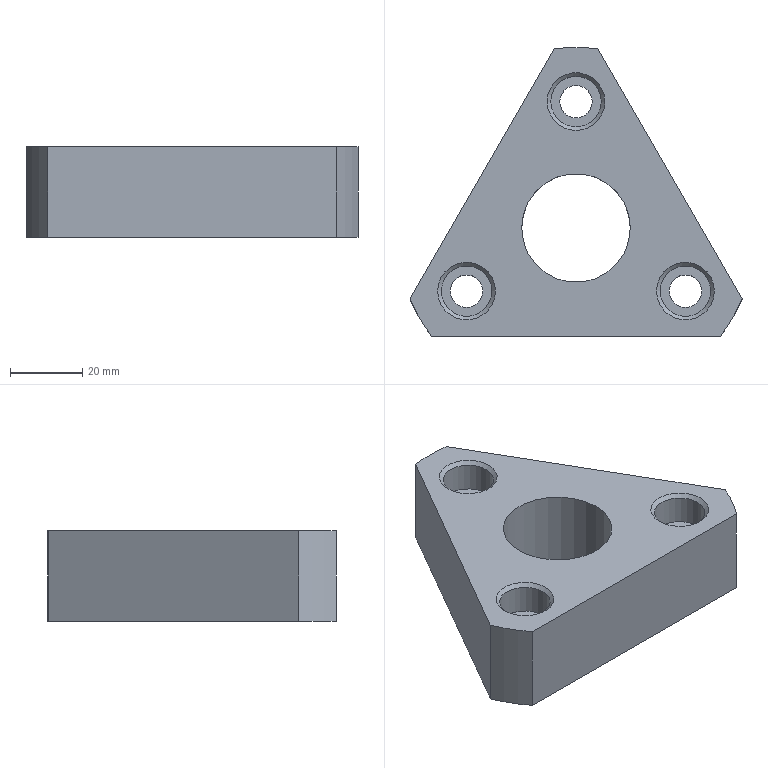NC program | NX | posted with a generic post | part box 91.962 x 80 x 25 mm
Lines 829 to 1659 of 11626:
(ZLEVEL_PROFILE_COPY , TOOL : D25R0.8)
N1632 T01 M6
N1634 G54
N1636 G17 G0 G90 X-0.726 Y-12.359 S1600 M3
N1638 G43 Z30. H1
N1640 Z1.
N1642 G94 G1 X-0.554 Y-12.412 Z0.991 F1000.
N1644 X-0.176 Y-12.436 Z0.971
N1646 X-0.153 Y-12.445 Z0.969
N1648 X-0.141 Y-12.441
N1650 X0.128 Z0.955
N1652 X0.136 Y-12.446 Z0.954
N1654 X0.157 Y-12.436 Z0.953
N1656 X0.354 Y-12.417 Z0.943
N1658 X1.218 Y-12.12 Z0.895
N1660 X2.118 Y-11.218 Z0.828
N1662 X2.308 Y-10.893 Z0.808
N1664 X2.414 Y-10.542 Z0.789
N1666 X2.436 Y-10.166 Z0.769
N1668 X2.446 Y-10.141 Z0.768
N1670 Y-9.859 Z0.753
N1672 X2.436 Y-9.839 Z0.752
N1674 X2.417 Y-9.644 Z0.742
N1676 X2.118 Y-8.782 Z0.694
N1678 X1.218 Y-7.88 Z0.627
N1680 X0.89 Y-7.69 Z0.607
N1682 X0.515 Y-7.581 Z0.587
N1684 X0.136 Y-7.563 Z0.567
N1686 Y-7.554 Z0.566
N1688 X0.128 Y-7.559
N1690 X-0.153 Y-7.555 Z0.551
N1692 X-0.171 Y-7.564 Z0.55
N1694 X-0.548 Y-7.587 Z0.53
N1696 X-0.892 Y-7.692 Z0.511
N1698 X-1.218 Y-7.882 Z0.492
N1700 X-2.118 Y-8.782 Z0.425
N1702 X-2.308 Y-9.105 Z0.405
N1704 X-2.419 Y-9.478 Z0.385
N1706 X-2.437 Y-9.852 Z0.365
N1708 X-2.446
N1710 Y-10.148 Z0.349
N1712 X-2.436 Y-10.167 Z0.348
N1714 X-2.414 Y-10.543 Z0.328
N1716 X-2.308 Y-10.893 Z0.309
N1718 X-2.118 Y-11.218 Z0.289
N1720 X-1.218 Y-12.118 Z0.223
N1722 X-0.892 Y-12.309 Z0.203
N1724 X-0.554 Y-12.412 Z0.184
N1726 X-0.176 Y-12.436 Z0.165
N1728 X-0.153 Y-12.445 Z0.163
N1730 X-0.141 Y-12.441
N1732 X0.128 Z0.149
N1734 X0.136 Y-12.446 Z0.148
N1736 X0.157 Y-12.436 Z0.147
N1738 X0.354 Y-12.417 Z0.137
N1740 X1.218 Y-12.12 Z0.089
N1742 X2.118 Y-11.218 Z0.022
N1744 X2.308 Y-10.893 Z0.002
N1746 X2.414 Y-10.542 Z-0.017
N1748 X2.436 Y-10.166 Z-0.037
N1750 X2.446 Y-10.141 Z-0.038
N1752 Y-9.859 Z-0.053
N1754 X2.436 Y-9.839 Z-0.054
N1756 X2.417 Y-9.644 Z-0.064
N1758 X2.118 Y-8.782 Z-0.112
N1760 X1.218 Y-7.88 Z-0.179
N1762 X0.89 Y-7.69 Z-0.199
N1764 X0.515 Y-7.581 Z-0.219
N1766 X0.136 Y-7.563 Z-0.239
N1768 Y-7.554 Z-0.24
N1770 X0.128 Y-7.559
N1772 X-0.153 Y-7.555 Z-0.255
N1774 X-0.171 Y-7.564 Z-0.256
N1776 X-0.548 Y-7.587 Z-0.276
N1778 X-0.892 Y-7.692 Z-0.295
N1780 X-1.218 Y-7.882 Z-0.314
N1782 X-1.668 Y-8.332 Z-0.348
N1784 X-2.118 Y-8.782 F1800.
N1786 G3 X-2.437 Y-9.852 R2.327
N1788 G1 X-2.446
N1790 Y-10.148
N1792 X-2.436 Y-10.167
N1794 G3 X-2.118 Y-11.218 R2.352
N1796 G1 X-1.218 Y-12.118
N1798 G3 X-0.176 Y-12.436 R2.371
N1800 G1 X-0.153 Y-12.445
N1802 X-0.141 Y-12.441
N1804 X0.128
N1806 X0.136 Y-12.446
N1808 X0.157 Y-12.436
N1810 X0.354 Y-12.417
N1812 X1.218 Y-12.12
N1814 X2.118 Y-11.218
N1816 G3 X2.436 Y-10.166 R2.356
N1818 G1 X2.446 Y-10.141
N1820 Y-9.859
N1822 X2.436 Y-9.839
N1824 X2.417 Y-9.644
N1826 X2.118 Y-8.782
N1828 X1.218 Y-7.88
N1830 G3 X0.136 Y-7.563 R2.383
N1832 G1 Y-7.554
N1834 X0.128 Y-7.559
N1836 X-0.153 Y-7.555
N1838 X-0.171 Y-7.564
N1840 G3 X-1.218 Y-7.882 R2.363
N1842 G1 X-1.668 Y-8.332
N1844 X-2.101 Y-8.765 Z-0.362
N1846 X-2.349 Y-9.322 Z-0.376
N1848 X-2.446 Y-9.917 Z-0.39
N1850 X-2.388 Y-10.524 Z-0.403
N1852 X-2.183 Y-11.1 Z-0.417
N1854 X-1.78 Y-11.556 Z-0.431
N1856 X-1.347 Y-11.989 Z-0.445
N1858 X-0.829 Y-12.3 Z-0.459
N1860 X-0.232 Y-12.432 Z-0.473
N1862 X0.373 Y-12.411 Z-0.487
N1864 X0.952 Y-12.212 Z-0.501
N1866 X1.452 Y-11.886 Z-0.515
N1868 X1.885 Y-11.452 Z-0.529
N1870 X2.246 Y-10.966 Z-0.543
N1872 X2.414 Y-10.379 Z-0.557
N1874 X2.43 Y-9.772 Z-0.57
N1876 X2.259 Y-9.187 Z-0.584
N1878 X1.988 Y-8.652 Z-0.598
N1880 X1.555 Y-8.218 Z-0.612
N1882 X1.099 Y-7.815 Z-0.626
N1884 X0.523 Y-7.613 Z-0.64
N1886 X-0.076 Y-7.556 Z-0.654
N1888 X-0.678 Y-7.651 Z-0.668
N1890 X-1.235 Y-7.899 Z-0.682
N1892 X-1.668 Y-8.332 Z-0.696
N1894 X-2.118 Y-8.782
N1896 G3 X-2.437 Y-9.852 R2.327
N1898 G1 X-2.446
N1900 Y-10.148
N1902 X-2.436 Y-10.167
N1904 G3 X-2.118 Y-11.218 R2.352
N1906 G1 X-1.218 Y-12.118
N1908 G3 X-0.176 Y-12.436 R2.371
N1910 G1 X-0.153 Y-12.445
N1912 X-0.141 Y-12.441
N1914 X0.128
N1916 X0.136 Y-12.446
N1918 X0.157 Y-12.436
N1920 X0.354 Y-12.417
N1922 X1.218 Y-12.12
N1924 X2.118 Y-11.218
N1926 G3 X2.436 Y-10.166 R2.356
N1928 G1 X2.446 Y-10.141
N1930 Y-9.859
N1932 X2.436 Y-9.839
N1934 X2.417 Y-9.644
N1936 X2.118 Y-8.782
N1938 X1.218 Y-7.88
N1940 G3 X0.136 Y-7.563 R2.383
N1942 G1 Y-7.554
N1944 X0.128 Y-7.559
N1946 X-0.153 Y-7.555
N1948 X-0.171 Y-7.564
N1950 G3 X-1.218 Y-7.882 R2.363
N1952 G1 X-1.668 Y-8.332
N1954 Z0.304
N1956 G0 X-0.553 Y-12.416
N1958 G1 X-0.153 Y-12.445 Z0.283 F1000.
N1960 X0.231 Y-12.469 Z0.263
N1962 X1.213 Y-12.163 Z0.209
N1964 X1.987 Y-11.484 Z0.155
N1966 X2.418 Y-10.55 Z0.101
N1968 X2.446 Y-10.141 Z0.08
N1970 X2.454 Y-10. Z0.073
N1972 X2.445 Y-9.838 Z0.064
N1974 X2.419 Y-9.455 Z0.044
N1976 X2.046 Y-8.598 Z-0.005
N1978 X1.381 Y-7.94 Z-0.054
N1980 X0.521 Y-7.575 Z-0.103
N1982 X0.136 Y-7.554 Z-0.123
N1984 X-0.008 Y-7.546 Z-0.131
N1986 X-0.172 Y-7.556 Z-0.139
N1988 X-0.555 Y-7.583 Z-0.16
N1990 X-1.46 Y-7.996 Z-0.212
N1992 X-2.004 Y-8.54 Z-0.252
N1994 X-2.422 Y-9.468 Z-0.305
N1996 X-2.446 Y-9.852 Z-0.326
N1998 X-2.454 Y-10. Z-0.333
N2000 X-2.444 Y-10.168 Z-0.342
N2002 X-2.418 Y-10.551 Z-0.362
N2004 X-2.051 Y-11.394 Z-0.41
N2006 X-1.402 Y-12.046 Z-0.459
N2008 X-0.56 Y-12.416 Z-0.507
N2010 X-0.153 Y-12.445 Z-0.528
N2012 X0.231 Y-12.469 Z-0.548
N2014 X1.213 Y-12.163 Z-0.602
N2016 X1.987 Y-11.484 Z-0.656
N2018 X2.418 Y-10.55 Z-0.71
N2020 X2.446 Y-10.141 Z-0.732
N2022 X2.454 Y-10. Z-0.739
N2024 X2.445 Y-9.838 Z-0.748
N2026 X2.419 Y-9.455 Z-0.768
N2028 X2.046 Y-8.598 Z-0.817
N2030 X1.381 Y-7.94 Z-0.866
N2032 X0.521 Y-7.575 Z-0.915
N2034 X0.136 Y-7.554 Z-0.935
N2036 X-0.008 Y-7.546 Z-0.942
N2038 X-0.172 Y-7.556 Z-0.951
N2040 X-0.555 Y-7.583 Z-0.971
N2042 X-1.46 Y-7.996 Z-1.023
N2044 X-1.732 Y-8.268 Z-1.043
N2046 G3 X-1.732 Y-11.732 R2.45 F1800.
N2048 X-1.732 Y-8.268 R-2.45
N2050 G1 X-1.963 Y-8.549 Z-1.052
N2052 X-2.088 Y-8.737 Z-1.057
N2054 X-2.25 Y-9.055 Z-1.065
N2056 X-2.332 Y-9.273 Z-1.07
N2058 X-2.402 Y-9.567 Z-1.077
N2060 X-2.438 Y-9.852 Z-1.084
N2062 X-2.442 Y-10.045 Z-1.088
N2064 X-2.437 Y-10.164 Z-1.091
N2066 X-2.368 Y-10.598 Z-1.101
N2068 X-2.291 Y-10.848 Z-1.107
N2070 X-2.115 Y-11.221 Z-1.116
N2072 X-1.958 Y-11.46 Z-1.122
N2074 X-1.688 Y-11.764 Z-1.132
N2076 X-1.467 Y-11.953 Z-1.138
N2078 X-1.121 Y-12.169 Z-1.148
N2080 X-0.856 Y-12.288 Z-1.154
N2082 X-0.445 Y-12.402 Z-1.164
N2084 X-0.152 Y-12.438 Z-1.17
N2086 X0.15 Z-1.177
N2088 X0.3 Y-12.423 Z-1.181
N2090 X0.402 Y-12.409 Z-1.183
N2092 X0.606 Y-12.366 Z-1.188
N2094 X0.897 Y-12.273 Z-1.195
N2096 X1.036 Y-12.212 Z-1.198
N2098 X1.127 Y-12.165 Z-1.2
N2100 X1.304 Y-12.063 Z-1.205
N2102 X1.559 Y-11.877 Z-1.212
N2104 X1.678 Y-11.774 Z-1.216
N2106 X1.747 Y-11.707 Z-1.218
N2108 X1.878 Y-11.562 Z-1.222
N2110 X2.14 Y-11.172 Z-1.233
N2112 X2.267 Y-10.908 Z-1.24
N2114 X2.348 Y-10.665 Z-1.246
N2116 X2.381 Y-10.54 Z-1.248
N2118 X2.407 Y-10.409 Z-1.252
N2120 X2.439 Y-10.141 Z-1.258
N2122 X2.446 Y-9.96 Z-1.262
N2124 X2.439 Y-9.859 Z-1.264
N2126 X2.362 Y-9.376 Z-1.275
N2128 X2.287 Y-9.15 Z-1.281
N2130 X2.103 Y-8.759 Z-1.29
N2132 X1.949 Y-8.532 Z-1.297
N2134 X1.669 Y-8.218 Z-1.306
N2136 X1.448 Y-8.036 Z-1.313
N2138 X1.092 Y-7.817 Z-1.322
N2140 X0.827 Y-7.704 Z-1.329
N2142 X0.619 Y-7.629 Z-1.334
N2144 X0.512 Y-7.604 Z-1.336
N2146 X0.387 Y-7.589 Z-1.339
N2148 X0.136 Y-7.564 Z-1.345
N2150 X-0.016 Y-7.56 Z-1.348
N2152 X-0.169 Y-7.556 Z-1.352
N2154 X-0.449 Y-7.6 Z-1.358
N2156 X-0.741 Y-7.675 Z-1.365
N2158 X-1.05 Y-7.797 Z-1.372
N2160 X-1.27 Y-7.914 Z-1.378
N2162 X-1.509 Y-8.082 Z-1.385
N2164 X-1.732 Y-8.268 Z-1.391
N2166 X-1.963 Y-8.549 Z-1.4
N2168 X-2.088 Y-8.737 Z-1.405
N2170 X-2.25 Y-9.055 Z-1.413
N2172 X-2.332 Y-9.273 Z-1.418
N2174 X-2.402 Y-9.567 Z-1.425
N2176 X-2.438 Y-9.852 Z-1.431
N2178 X-2.442 Y-10.045 Z-1.436
N2180 X-2.437 Y-10.164 Z-1.439
N2182 X-2.368 Y-10.598 Z-1.449
N2184 X-2.291 Y-10.848 Z-1.454
N2186 X-2.115 Y-11.221 Z-1.464
N2188 X-1.958 Y-11.46 Z-1.47
N2190 X-1.688 Y-11.764 Z-1.479
N2192 X-1.467 Y-11.953 Z-1.486
N2194 X-1.121 Y-12.169 Z-1.495
N2196 X-0.856 Y-12.288 Z-1.502
N2198 X-0.445 Y-12.402 Z-1.512
N2200 X-0.152 Y-12.438 Z-1.518
N2202 X0.15 Z-1.525
N2204 X0.3 Y-12.423 Z-1.529
N2206 X0.402 Y-12.409 Z-1.531
N2208 X0.606 Y-12.366 Z-1.536
N2210 X0.897 Y-12.273 Z-1.543
N2212 X1.036 Y-12.212 Z-1.546
N2214 X1.127 Y-12.165 Z-1.548
N2216 X1.304 Y-12.063 Z-1.553
N2218 X1.559 Y-11.877 Z-1.56
N2220 X1.678 Y-11.774 Z-1.564
N2222 X1.747 Y-11.707 Z-1.566
N2224 X1.878 Y-11.562 Z-1.57
N2226 X2.14 Y-11.172 Z-1.581
N2228 X2.267 Y-10.908 Z-1.588
N2230 X2.348 Y-10.665 Z-1.593
N2232 X2.381 Y-10.54 Z-1.596
N2234 X2.407 Y-10.409 Z-1.599
N2236 X2.439 Y-10.141 Z-1.605
N2238 X2.446 Y-9.96 Z-1.61
N2240 X2.439 Y-9.859 Z-1.612
N2242 X2.362 Y-9.376 Z-1.623
N2244 X2.287 Y-9.15 Z-1.628
N2246 X2.103 Y-8.759 Z-1.638
N2248 X1.949 Y-8.532 Z-1.644
N2250 X1.669 Y-8.218 Z-1.654
N2252 X1.448 Y-8.036 Z-1.66
N2254 X1.092 Y-7.817 Z-1.67
N2256 X0.827 Y-7.704 Z-1.676
N2258 X0.619 Y-7.629 Z-1.681
N2260 X0.512 Y-7.604 Z-1.684
N2262 X0.387 Y-7.589 Z-1.687
N2264 X0.136 Y-7.564 Z-1.693
N2266 X-0.016 Y-7.56 Z-1.696
N2268 X-0.169 Y-7.556 Z-1.699
N2270 X-0.449 Y-7.6 Z-1.706
N2272 X-0.741 Y-7.675 Z-1.713
N2274 X-1.05 Y-7.797 Z-1.72
N2276 X-1.27 Y-7.914 Z-1.726
N2278 X-1.509 Y-8.082 Z-1.733
N2280 X-1.732 Y-8.268 Z-1.739
N2282 X-1.963 Y-8.549 Z-1.747
N2284 X-2.088 Y-8.737 Z-1.753
N2286 X-2.25 Y-9.055 Z-1.761
N2288 X-2.332 Y-9.273 Z-1.766
N2290 X-2.402 Y-9.567 Z-1.773
N2292 X-2.438 Y-9.852 Z-1.779
N2294 X-2.442 Y-10.045 Z-1.784
N2296 X-2.437 Y-10.164 Z-1.786
N2298 X-2.368 Y-10.598 Z-1.796
N2300 X-2.291 Y-10.848 Z-1.802
N2302 X-2.115 Y-11.221 Z-1.812
N2304 X-1.958 Y-11.46 Z-1.818
N2306 X-1.688 Y-11.764 Z-1.827
N2308 X-1.467 Y-11.953 Z-1.834
N2310 X-1.121 Y-12.169 Z-1.843
N2312 X-0.856 Y-12.288 Z-1.85
N2314 X-0.445 Y-12.402 Z-1.859
N2316 X-0.152 Y-12.438 Z-1.866
N2318 X0.15 Z-1.873
N2320 X0.3 Y-12.423 Z-1.876
N2322 X0.402 Y-12.409 Z-1.879
N2324 X0.606 Y-12.366 Z-1.883
N2326 X0.897 Y-12.273 Z-1.89
N2328 X1.036 Y-12.212 Z-1.894
N2330 X1.127 Y-12.165 Z-1.896
N2332 X1.304 Y-12.063 Z-1.901
N2334 X1.559 Y-11.877 Z-1.908
N2336 X1.678 Y-11.774 Z-1.911
N2338 X1.747 Y-11.707 Z-1.914
N2340 X1.878 Y-11.562 Z-1.918
N2342 X2.14 Y-11.172 Z-1.929
N2344 X2.267 Y-10.908 Z-1.935
N2346 X2.348 Y-10.665 Z-1.941
N2348 X2.381 Y-10.54 Z-1.944
N2350 X2.407 Y-10.409 Z-1.947
N2352 X2.439 Y-10.141 Z-1.953
N2354 X2.445 Y-9.96 Z-1.957
N2356 X2.439 Y-9.859 Z-1.96
N2358 X2.362 Y-9.376 Z-1.971
N2360 X2.287 Y-9.15 Z-1.976
N2362 X2.103 Y-8.759 Z-1.986
N2364 X1.949 Y-8.532 Z-1.992
N2366 X1.669 Y-8.218 Z-2.002
N2368 X1.448 Y-8.036 Z-2.008
N2370 X1.092 Y-7.817 Z-2.018
N2372 X0.827 Y-7.704 Z-2.024
N2374 X0.619 Y-7.629 Z-2.029
N2376 X0.389 Y-7.581 Z-2.035
N2378 X0.136 Y-7.564 Z-2.04
N2380 X-0.017 Y-7.55 Z-2.044
N2382 X-0.169 Y-7.556 Z-2.047
N2384 X-0.497 Y-7.601 Z-2.055
N2386 X-0.741 Y-7.675 Z-2.061
N2388 X-1.087 Y-7.813 Z-2.069
N2390 X-1.27 Y-7.914 Z-2.074
N2392 X-1.509 Y-8.082 Z-2.08
N2394 X-1.732 Y-8.268 Z-2.087
N2396 X-1.963 Y-8.549 Z-2.095
N2398 X-2.088 Y-8.737 Z-2.1
N2400 X-2.25 Y-9.055 Z-2.108
N2402 X-2.332 Y-9.273 Z-2.114
N2404 X-2.402 Y-9.567 Z-2.121
N2406 X-2.438 Y-9.852 Z-2.127
N2408 X-2.442 Y-10.045 Z-2.131
N2410 X-2.437 Y-10.164 Z-2.134
N2412 X-2.368 Y-10.598 Z-2.144
N2414 X-2.291 Y-10.848 Z-2.15
N2416 X-2.115 Y-11.221 Z-2.159
N2418 X-1.958 Y-11.46 Z-2.166
N2420 X-1.688 Y-11.764 Z-2.175
N2422 X-1.467 Y-11.953 Z-2.182
N2424 X-1.121 Y-12.169 Z-2.191
N2426 X-0.856 Y-12.288 Z-2.198
N2428 X-0.445 Y-12.402 Z-2.207
N2430 X-0.152 Y-12.438 Z-2.214
N2432 X0.15 Z-2.221
N2434 X0.3 Y-12.423 Z-2.224
N2436 X0.402 Y-12.409 Z-2.227
N2438 X0.606 Y-12.366 Z-2.231
N2440 X0.897 Y-12.273 Z-2.238
N2442 X1.036 Y-12.212 Z-2.242
N2444 X1.127 Y-12.165 Z-2.244
N2446 X1.304 Y-12.063 Z-2.249
N2448 X1.559 Y-11.877 Z-2.256
N2450 X1.678 Y-11.774 Z-2.259
N2452 X1.747 Y-11.707 Z-2.261
N2454 X1.878 Y-11.562 Z-2.266
N2456 X2.14 Y-11.172 Z-2.277
N2458 X2.267 Y-10.908 Z-2.283
N2460 X2.348 Y-10.665 Z-2.289
N2462 X2.381 Y-10.54 Z-2.292
N2464 X2.407 Y-10.409 Z-2.295
N2466 X2.439 Y-10.141 Z-2.301
N2468 X2.445 Y-9.96 Z-2.305
N2470 X2.439 Y-9.859 Z-2.308
N2472 X2.362 Y-9.376 Z-2.319
N2474 X2.287 Y-9.15 Z-2.324
N2476 X2.103 Y-8.759 Z-2.334
N2478 X1.949 Y-8.532 Z-2.34
N2480 X1.669 Y-8.218 Z-2.35
N2482 X1.448 Y-8.036 Z-2.356
N2484 X1.092 Y-7.817 Z-2.366
N2486 X0.827 Y-7.704 Z-2.372
N2488 X0.619 Y-7.629 Z-2.377
N2490 X0.389 Y-7.581 Z-2.382
N2492 X0.136 Y-7.564 Z-2.388
N2494 X-0.017 Y-7.55 Z-2.392
N2496 X-0.169 Y-7.556 Z-2.395
N2498 X-0.497 Y-7.601 Z-2.403
N2500 X-0.741 Y-7.675 Z-2.408
N2502 X-1.087 Y-7.813 Z-2.417
N2504 X-1.27 Y-7.914 Z-2.422
N2506 X-1.509 Y-8.082 Z-2.428
N2508 X-1.732 Y-8.268 Z-2.435
N2510 X-1.963 Y-8.549 Z-2.443
N2512 X-2.088 Y-8.737 Z-2.448
N2514 X-2.25 Y-9.055 Z-2.456
N2516 X-2.332 Y-9.273 Z-2.462
N2518 X-2.402 Y-9.567 Z-2.468
N2520 X-2.438 Y-9.852 Z-2.475
N2522 X-2.442 Y-10.045 Z-2.479
N2524 X-2.437 Y-10.164 Z-2.482
N2526 X-2.368 Y-10.598 Z-2.492
N2528 X-2.291 Y-10.848 Z-2.498
N2530 X-2.115 Y-11.221 Z-2.507
N2532 X-1.958 Y-11.46 Z-2.514
N2534 X-1.688 Y-11.764 Z-2.523
N2536 X-1.467 Y-11.953 Z-2.53
N2538 X-1.121 Y-12.169 Z-2.539
N2540 X-0.856 Y-12.288 Z-2.545
N2542 X-0.445 Y-12.402 Z-2.555
N2544 X-0.152 Y-12.438 Z-2.562
N2546 X0.15 Z-2.569
N2548 X0.3 Y-12.423 Z-2.572
N2550 X0.402 Y-12.409 Z-2.574
N2552 X0.606 Y-12.366 Z-2.579
N2554 X0.897 Y-12.273 Z-2.586
N2556 X1.036 Y-12.212 Z-2.589
N2558 X1.127 Y-12.165 Z-2.592
N2560 X1.304 Y-12.063 Z-2.596
N2562 X1.559 Y-11.877 Z-2.604
N2564 X1.678 Y-11.774 Z-2.607
N2566 X1.747 Y-11.707 Z-2.609
N2568 X1.878 Y-11.562 Z-2.614
N2570 X2.14 Y-11.172 Z-2.624
N2572 X2.267 Y-10.908 Z-2.631
N2574 X2.348 Y-10.665 Z-2.637
N2576 X2.381 Y-10.54 Z-2.64
N2578 X2.407 Y-10.409 Z-2.643
N2580 X2.439 Y-10.141 Z-2.649
N2582 X2.445 Y-9.96 Z-2.653
N2584 X2.439 Y-9.859 Z-2.655
N2586 X2.362 Y-9.376 Z-2.666
N2588 X2.287 Y-9.15 Z-2.672
N2590 X2.103 Y-8.759 Z-2.682
N2592 X1.949 Y-8.532 Z-2.688
N2594 X1.669 Y-8.218 Z-2.697
N2596 X1.448 Y-8.036 Z-2.704
N2598 X1.093 Y-7.817 Z-2.713
N2600 X0.827 Y-7.704 Z-2.72
N2602 X0.619 Y-7.629 Z-2.725
N2604 X0.389 Y-7.581 Z-2.73
N2606 X0.136 Y-7.564 Z-2.736
N2608 X-0.017 Y-7.55 Z-2.739
N2610 X-0.169 Y-7.556 Z-2.743
N2612 X-0.497 Y-7.601 Z-2.75
N2614 X-0.741 Y-7.675 Z-2.756
N2616 X-1.087 Y-7.813 Z-2.765
N2618 X-1.27 Y-7.914 Z-2.769
N2620 X-1.509 Y-8.082 Z-2.776
N2622 X-1.732 Y-8.268 Z-2.783
N2624 X-1.963 Y-8.549 Z-2.791
N2626 X-2.088 Y-8.737 Z-2.796
N2628 X-2.25 Y-9.055 Z-2.804
N2630 X-2.332 Y-9.273 Z-2.809
N2632 X-2.402 Y-9.567 Z-2.816
N2634 X-2.438 Y-9.852 Z-2.823
N2636 X-2.442 Y-10.045 Z-2.827
N2638 X-2.437 Y-10.164 Z-2.83
N2640 X-2.368 Y-10.598 Z-2.84
N2642 X-2.291 Y-10.848 Z-2.846
N2644 X-2.115 Y-11.221 Z-2.855
N2646 X-1.958 Y-11.46 Z-2.862
N2648 X-1.688 Y-11.764 Z-2.871
N2650 X-1.467 Y-11.953 Z-2.877
N2652 X-1.121 Y-12.169 Z-2.887
N2654 X-0.856 Y-12.288 Z-2.893
N2656 X-0.445 Y-12.402 Z-2.903
N2658 X-0.152 Y-12.438 Z-2.91
N2660 X0.3 Y-12.423 Z-2.92
N2662 X0.606 Y-12.366 Z-2.927
N2664 X0.885 Y-12.275 Z-2.934
N2666 X1.02 Y-12.219 Z-2.937
N2668 X1.117 Y-12.172 Z-2.939
N2670 X1.304 Y-12.063 Z-2.944
N2672 X1.562 Y-11.875 Z-2.951
N2674 X1.681 Y-11.771 Z-2.955
N2676 X1.749 Y-11.704 Z-2.957
N2678 X1.878 Y-11.562 Z-2.962
N2680 X2.141 Y-11.171 Z-2.972
N2682 X2.267 Y-10.908 Z-2.979
N2684 X2.348 Y-10.664 Z-2.985
N2686 X2.381 Y-10.54 Z-2.988
N2688 X2.407 Y-10.409 Z-2.991
N2690 X2.439 Y-10.141 Z-2.997
N2692 X2.445 Y-9.96 Z-3.001
N2694 X2.439 Y-9.859 Z-3.003
N2696 X2.362 Y-9.376 Z-3.014
N2698 X2.287 Y-9.15 Z-3.02
N2700 X2.103 Y-8.759 Z-3.029
N2702 X1.949 Y-8.532 Z-3.036
N2704 X1.669 Y-8.218 Z-3.045
N2706 X1.448 Y-8.036 Z-3.052
N2708 X1.093 Y-7.817 Z-3.061
N2710 X0.827 Y-7.704 Z-3.068
N2712 X0.619 Y-7.629 Z-3.073
N2714 X0.389 Y-7.581 Z-3.078
N2716 X0.136 Y-7.564 Z-3.084
N2718 X-0.017 Y-7.55 Z-3.087
N2720 X-0.169 Y-7.556 Z-3.091
N2722 X-0.497 Y-7.601 Z-3.098
N2724 X-0.741 Y-7.675 Z-3.104
N2726 X-1.087 Y-7.814 Z-3.112
N2728 X-1.27 Y-7.914 Z-3.117
N2730 X-1.509 Y-8.082 Z-3.124
N2732 X-1.732 Y-8.268 Z-3.13
N2734 X-1.963 Y-8.549 Z-3.139
N2736 X-2.088 Y-8.737 Z-3.144
N2738 X-2.25 Y-9.055 Z-3.152
N2740 X-2.332 Y-9.273 Z-3.157
N2742 X-2.402 Y-9.567 Z-3.164
N2744 X-2.438 Y-9.852 Z-3.171
N2746 X-2.442 Y-10.045 Z-3.175
N2748 X-2.437 Y-10.164 Z-3.178
N2750 X-2.368 Y-10.598 Z-3.188
N2752 X-2.291 Y-10.848 Z-3.194
N2754 X-2.115 Y-11.221 Z-3.203
N2756 X-1.958 Y-11.46 Z-3.209
N2758 X-1.688 Y-11.764 Z-3.219
N2760 X-1.467 Y-11.953 Z-3.225
N2762 X-1.121 Y-12.169 Z-3.234
N2764 X-0.856 Y-12.288 Z-3.241
N2766 X-0.445 Y-12.402 Z-3.251
N2768 X-0.152 Y-12.438 Z-3.257
N2770 X0.3 Y-12.423 Z-3.268
N2772 X0.606 Y-12.366 Z-3.275
N2774 X0.885 Y-12.275 Z-3.281
N2776 X1.02 Y-12.219 Z-3.285
N2778 X1.117 Y-12.172 Z-3.287
N2780 X1.304 Y-12.063 Z-3.292
N2782 X1.562 Y-11.875 Z-3.299
N2784 X1.681 Y-11.771 Z-3.303
N2786 X1.749 Y-11.704 Z-3.305
N2788 X1.878 Y-11.562 Z-3.309
N2790 X2.141 Y-11.171 Z-3.32
N2792 X2.267 Y-10.908 Z-3.327
N2794 X2.348 Y-10.664 Z-3.333
N2796 X2.381 Y-10.54 Z-3.335
N2798 X2.407 Y-10.409 Z-3.338
N2800 X2.439 Y-10.141 Z-3.345
N2802 X2.445 Y-9.96 Z-3.349
N2804 X2.439 Y-9.859 Z-3.351
N2806 X2.362 Y-9.376 Z-3.362
N2808 X2.287 Y-9.15 Z-3.367
N2810 X2.103 Y-8.759 Z-3.377
N2812 X1.949 Y-8.532 Z-3.384
N2814 X1.669 Y-8.218 Z-3.393
N2816 X1.448 Y-8.036 Z-3.4
N2818 X1.093 Y-7.817 Z-3.409
N2820 X0.827 Y-7.704 Z-3.416
N2822 X0.619 Y-7.629 Z-3.421
N2824 X0.389 Y-7.581 Z-3.426
N2826 X0.136 Y-7.564 Z-3.432
N2828 X-0.017 Y-7.55 Z-3.435
N2830 X-0.169 Y-7.556 Z-3.439
N2832 X-0.497 Y-7.601 Z-3.446
N2834 X-0.741 Y-7.675 Z-3.452
N2836 X-1.087 Y-7.814 Z-3.46
N2838 X-1.27 Y-7.914 Z-3.465
N2840 X-1.509 Y-8.082 Z-3.472
N2842 X-1.732 Y-8.268 Z-3.478
N2844 X-1.963 Y-8.549 Z-3.486
N2846 X-2.088 Y-8.737 Z-3.492
N2848 X-2.25 Y-9.055 Z-3.5
N2850 X-2.332 Y-9.273 Z-3.505
N2852 X-2.402 Y-9.567 Z-3.512
N2854 X-2.438 Y-9.852 Z-3.518
N2856 X-2.442 Y-10.045 Z-3.523
N2858 X-2.437 Y-10.164 Z-3.526
N2860 X-2.368 Y-10.598 Z-3.535
N2862 X-2.291 Y-10.848 Z-3.541
N2864 X-2.115 Y-11.221 Z-3.551
N2866 X-1.958 Y-11.46 Z-3.557
N2868 X-1.688 Y-11.764 Z-3.566
N2870 X-1.467 Y-11.953 Z-3.573
N2872 X-1.121 Y-12.169 Z-3.582
N2874 X-0.856 Y-12.288 Z-3.589
N2876 X-0.445 Y-12.402 Z-3.599
N2878 X-0.152 Y-12.438 Z-3.605
N2880 X0.3 Y-12.423 Z-3.616
N2882 X0.606 Y-12.366 Z-3.623
N2884 X0.885 Y-12.275 Z-3.629
N2886 X1.02 Y-12.219 Z-3.633
N2888 X1.117 Y-12.172 Z-3.635
N2890 X1.304 Y-12.063 Z-3.64
N2892 X1.562 Y-11.875 Z-3.647
N2894 X1.681 Y-11.771 Z-3.651
N2896 X1.749 Y-11.704 Z-3.653
N2898 X1.878 Y-11.562 Z-3.657
N2900 X2.141 Y-11.171 Z-3.668
N2902 X2.267 Y-10.908 Z-3.675
N2904 X2.348 Y-10.664 Z-3.68
N2906 X2.381 Y-10.54 Z-3.683
N2908 X2.407 Y-10.409 Z-3.686
N2910 X2.439 Y-10.141 Z-3.692
N2912 X2.445 Y-9.96 Z-3.697
N2914 X2.439 Y-9.859 Z-3.699
N2916 X2.362 Y-9.376 Z-3.71
N2918 X2.287 Y-9.15 Z-3.715
N2920 X2.103 Y-8.759 Z-3.725
N2922 X1.949 Y-8.532 Z-3.731
N2924 X1.669 Y-8.218 Z-3.741
N2926 X1.448 Y-8.036 Z-3.747
N2928 X1.093 Y-7.817 Z-3.757
N2930 X0.827 Y-7.704 Z-3.763
N2932 X0.619 Y-7.629 Z-3.768
N2934 X0.389 Y-7.581 Z-3.774
N2936 X0.136 Y-7.564 Z-3.779
N2938 X-0.017 Y-7.55 Z-3.783
N2940 X-0.169 Y-7.556 Z-3.786
N2942 X-0.497 Y-7.601 Z-3.794
N2944 X-0.741 Y-7.675 Z-3.8
N2946 X-1.087 Y-7.814 Z-3.808
N2948 X-1.27 Y-7.914 Z-3.813
N2950 X-1.509 Y-8.082 Z-3.819
N2952 X-1.732 Y-8.268 Z-3.826
N2954 X-1.963 Y-8.549 Z-3.834
N2956 X-2.088 Y-8.737 Z-3.839
N2958 X-2.25 Y-9.055 Z-3.848
N2960 X-2.332 Y-9.273 Z-3.853
N2962 X-2.402 Y-9.567 Z-3.86
N2964 X-2.438 Y-9.852 Z-3.866
N2966 X-2.442 Y-10.045 Z-3.871
N2968 X-2.437 Y-10.164 Z-3.873
N2970 X-2.368 Y-10.598 Z-3.883
N2972 X-2.291 Y-10.848 Z-3.889
N2974 X-2.115 Y-11.221 Z-3.899
N2976 X-1.958 Y-11.46 Z-3.905
N2978 X-1.688 Y-11.764 Z-3.914
N2980 X-1.467 Y-11.953 Z-3.921
N2982 X-1.121 Y-12.169 Z-3.93
N2984 X-0.856 Y-12.288 Z-3.937
N2986 X-0.445 Y-12.402 Z-3.946
N2988 X-0.152 Y-12.438 Z-3.953
N2990 X0.3 Y-12.423 Z-3.963
N2992 X0.606 Y-12.366 Z-3.97
N2994 X0.885 Y-12.275 Z-3.977
N2996 X1.02 Y-12.219 Z-3.98
N2998 X1.117 Y-12.172 Z-3.983
N3000 X1.304 Y-12.063 Z-3.988
N3002 X1.562 Y-11.875 Z-3.995
N3004 X1.681 Y-11.771 Z-3.999
N3006 X1.749 Y-11.704 Z-4.001
N3008 X1.878 Y-11.562 Z-4.005
N3010 X2.141 Y-11.171 Z-4.016
N3012 X2.267 Y-10.908 Z-4.022
N3014 X2.348 Y-10.664 Z-4.028
N3016 X2.381 Y-10.54 Z-4.031
N3018 X2.407 Y-10.409 Z-4.034
N3020 X2.439 Y-10.141 Z-4.04
N3022 X2.445 Y-9.96 Z-4.044
N3024 X2.439 Y-9.859 Z-4.047
N3026 X2.362 Y-9.376 Z-4.058
N3028 X2.287 Y-9.15 Z-4.063
N3030 X2.103 Y-8.759 Z-4.073
N3032 X1.949 Y-8.532 Z-4.079
N3034 X1.669 Y-8.218 Z-4.089
N3036 X1.448 Y-8.036 Z-4.095
N3038 X1.093 Y-7.817 Z-4.105
N3040 X0.827 Y-7.704 Z-4.111
N3042 X0.619 Y-7.629 Z-4.116
N3044 X0.389 Y-7.581 Z-4.122
N3046 X0.136 Y-7.564 Z-4.127
N3048 X-0.017 Y-7.55 Z-4.131
N3050 X-0.169 Y-7.556 Z-4.134
N3052 X-0.497 Y-7.601 Z-4.142
N3054 X-0.741 Y-7.675 Z-4.147
N3056 X-1.087 Y-7.814 Z-4.156
N3058 X-1.27 Y-7.914 Z-4.161
N3060 X-1.509 Y-8.082 Z-4.167
N3062 X-1.732 Y-8.268 Z-4.174
N3064 X-1.963 Y-8.549 Z-4.182
N3066 X-2.088 Y-8.737 Z-4.187
N3068 X-2.25 Y-9.055 Z-4.195
N3070 X-2.332 Y-9.273 Z-4.201
N3072 X-2.402 Y-9.567 Z-4.208
N3074 X-2.438 Y-9.852 Z-4.214
N3076 X-2.442 Y-10.045 Z-4.218
N3078 X-2.437 Y-10.164 Z-4.221
N3080 X-2.368 Y-10.598 Z-4.231
N3082 X-2.291 Y-10.848 Z-4.237
N3084 X-2.115 Y-11.221 Z-4.246
N3086 X-1.958 Y-11.46 Z-4.253
N3088 X-1.688 Y-11.764 Z-4.262
N3090 X-1.467 Y-11.953 Z-4.269
N3092 X-1.121 Y-12.169 Z-4.278
N3094 X-0.856 Y-12.288 Z-4.285
N3096 X-0.445 Y-12.402 Z-4.294
N3098 X-0.152 Y-12.438 Z-4.301
N3100 X0.3 Y-12.423 Z-4.311
N3102 X0.606 Y-12.366 Z-4.318
N3104 X0.885 Y-12.275 Z-4.325
N3106 X1.02 Y-12.219 Z-4.328
N3108 X1.117 Y-12.172 Z-4.331
N3110 X1.304 Y-12.063 Z-4.336
N3112 X1.562 Y-11.875 Z-4.343
N3114 X1.681 Y-11.771 Z-4.346
N3116 X1.749 Y-11.704 Z-4.349
N3118 X1.878 Y-11.562 Z-4.353
N3120 X2.141 Y-11.171 Z-4.364
N3122 X2.267 Y-10.908 Z-4.37
N3124 X2.348 Y-10.664 Z-4.376
N3126 X2.381 Y-10.54 Z-4.379
N3128 X2.407 Y-10.409 Z-4.382
N3130 X2.439 Y-10.141 Z-4.388
N3132 X2.445 Y-9.96 Z-4.392
N3134 X2.439 Y-9.859 Z-4.394
N3136 X2.362 Y-9.376 Z-4.406
N3138 X2.287 Y-9.15 Z-4.411
N3140 X2.103 Y-8.759 Z-4.421
N3142 X1.949 Y-8.532 Z-4.427
N3144 X1.669 Y-8.218 Z-4.437
N3146 X1.448 Y-8.036 Z-4.443
N3148 X1.093 Y-7.817 Z-4.453
N3150 X0.827 Y-7.704 Z-4.459
N3152 X0.619 Y-7.629 Z-4.464
N3154 X0.389 Y-7.581 Z-4.469
N3156 X0.136 Y-7.564 Z-4.475
N3158 X-0.017 Y-7.55 Z-4.479
N3160 X-0.169 Y-7.556 Z-4.482
N3162 X-0.497 Y-7.601 Z-4.49
N3164 X-0.741 Y-7.675 Z-4.495
N3166 X-1.087 Y-7.814 Z-4.504
N3168 X-1.27 Y-7.914 Z-4.509
N3170 X-1.509 Y-8.082 Z-4.515
N3172 X-1.732 Y-8.268 Z-4.522
N3174 X-1.963 Y-8.549 Z-4.53
N3176 X-2.088 Y-8.737 Z-4.535
N3178 X-2.25 Y-9.055 Z-4.543
N3180 X-2.332 Y-9.273 Z-4.549
N3182 X-2.402 Y-9.567 Z-4.555
N3184 X-2.438 Y-9.852 Z-4.562
N3186 X-2.442 Y-10.045 Z-4.566
N3188 X-2.437 Y-10.164 Z-4.569
N3190 X-2.368 Y-10.598 Z-4.579
N3192 X-2.291 Y-10.848 Z-4.585
N3194 X-2.115 Y-11.221 Z-4.594
N3196 X-1.958 Y-11.46 Z-4.601
N3198 X-1.688 Y-11.764 Z-4.61
N3200 X-1.467 Y-11.953 Z-4.617
N3202 X-1.121 Y-12.169 Z-4.626
N3204 X-0.856 Y-12.288 Z-4.632
N3206 X-0.445 Y-12.402 Z-4.642
N3208 X-0.152 Y-12.438 Z-4.649
N3210 X0.3 Y-12.423 Z-4.659
N3212 X0.606 Y-12.366 Z-4.666
N3214 X0.885 Y-12.275 Z-4.673
N3216 X1.02 Y-12.219 Z-4.676
N3218 X1.117 Y-12.172 Z-4.678
N3220 X1.304 Y-12.063 Z-4.683
N3222 X1.562 Y-11.875 Z-4.691
N3224 X1.681 Y-11.771 Z-4.694
N3226 X1.749 Y-11.704 Z-4.696
N3228 X1.877 Y-11.562 Z-4.701
N3230 X2.141 Y-11.171 Z-4.711
N3232 X2.267 Y-10.908 Z-4.718
N3234 X2.348 Y-10.664 Z-4.724
N3236 X2.381 Y-10.54 Z-4.727
N3238 X2.407 Y-10.409 Z-4.73
N3240 X2.439 Y-10.141 Z-4.736
N3242 X2.445 Y-9.96 Z-4.74
N3244 X2.439 Y-9.859 Z-4.742
N3246 X2.362 Y-9.377 Z-4.753
N3248 X2.287 Y-9.15 Z-4.759
N3250 X2.103 Y-8.759 Z-4.769
N3252 X1.949 Y-8.532 Z-4.775
N3254 X1.669 Y-8.218 Z-4.784
N3256 X1.448 Y-8.036 Z-4.791
N3258 X1.093 Y-7.817 Z-4.8
N3260 X0.827 Y-7.704 Z-4.807
N3262 X0.619 Y-7.629 Z-4.812
N3264 X0.389 Y-7.581 Z-4.817
N3266 X0.136 Y-7.564 Z-4.823
N3268 X-0.017 Y-7.55 Z-4.826
N3270 X-0.169 Y-7.556 Z-4.83
N3272 X-0.497 Y-7.601 Z-4.837
N3274 X-0.741 Y-7.675 Z-4.843
N3276 X-1.087 Y-7.814 Z-4.852
N3278 X-1.27 Y-7.914 Z-4.856
N3280 X-1.509 Y-8.082 Z-4.863
N3282 X-1.732 Y-8.268 Z-4.87
N3284 X-1.963 Y-8.549 Z-4.878
N3286 X-2.088 Y-8.737 Z-4.883